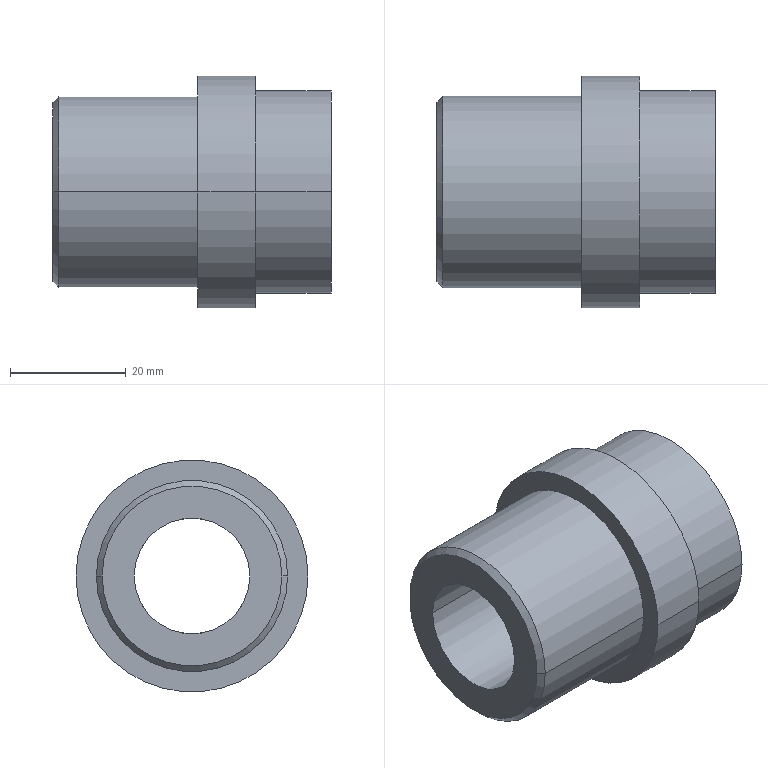Part | SolidWorks | features HoleWzd 1, ICE 1, Revolution 1 | 1 solid | 18 faces | box 48 x 40 x 40 mm | volume 30975 mm3 | cylinder 10 | cone 4 | plane 4 | commonest cylinder face diameters 20 x2 20.5 x2 33 x2 35 x2 40 x2
STEP:
#1=CARTESIAN_POINT('',(-22.,0.,10.25));
#2=VERTEX_POINT('',#1);
#3=CARTESIAN_POINT('',(-22.,0.,-10.25));
#4=VERTEX_POINT('',#3);
#5=CARTESIAN_POINT('',(-22.,0.,0.));
#6=DIRECTION('',(1.,0.,0.));
#7=DIRECTION('',(0.,0.,-1.));
#8=AXIS2_PLACEMENT_3D('',#5,#6,#7);
#9=CIRCLE('',#8,10.25);
#10=EDGE_CURVE('',#2,#4,#9,.T.);
#11=ORIENTED_EDGE('',*,*,#10,.F.);
#12=CARTESIAN_POINT('',(0.,0.,10.25));
#13=VERTEX_POINT('',#12);
#14=CARTESIAN_POINT('',(0.,0.,10.25));
#15=DIRECTION('',(1.,0.,0.));
#16=VECTOR('',#15,1000.);
#17=LINE('',#14,#16);
#18=EDGE_CURVE('',#2,#13,#17,.T.);
#19=ORIENTED_EDGE('',*,*,#18,.T.);
#20=CARTESIAN_POINT('',(0.,0.,-10.25));
#21=VERTEX_POINT('',#20);
#22=CARTESIAN_POINT('',(0.,0.,0.));
#23=DIRECTION('',(1.,0.,0.));
#24=DIRECTION('',(0.,0.,-1.));
#25=AXIS2_PLACEMENT_3D('',#22,#23,#24);
#26=CIRCLE('',#25,10.25);
#27=EDGE_CURVE('',#13,#21,#26,.T.);
#28=ORIENTED_EDGE('',*,*,#27,.T.);
#29=CARTESIAN_POINT('',(0.,0.,-10.25));
#30=DIRECTION('',(1.,0.,0.));
#31=VECTOR('',#30,1000.);
#32=LINE('',#29,#31);
#33=EDGE_CURVE('',#4,#21,#32,.T.);
#34=ORIENTED_EDGE('',*,*,#33,.F.);
#35=EDGE_LOOP('',(#11,#19,#28,#34));
#36=FACE_OUTER_BOUND('',#35,.T.);
#37=CARTESIAN_POINT('',(0.,0.,0.));
#38=DIRECTION('',(1.,0.,0.));
#39=DIRECTION('',(0.,0.,-1.));
#40=AXIS2_PLACEMENT_3D('',#37,#38,#39);
#41=CYLINDRICAL_SURFACE('',#40,10.25);
#42=ADVANCED_FACE('',(#36),#41,.F.);
#43=CARTESIAN_POINT('',(-22.15,0.,10.));
#44=VERTEX_POINT('',#43);
#45=CARTESIAN_POINT('',(-22.15,-10.,0.));
#46=VERTEX_POINT('',#45);
#47=CARTESIAN_POINT('',(-22.15,0.,0.));
#48=DIRECTION('',(1.,0.,0.));
#49=DIRECTION('',(0.,0.,-1.));
#50=AXIS2_PLACEMENT_3D('',#47,#48,#49);
#51=CIRCLE('',#50,10.);
#52=EDGE_CURVE('',#44,#46,#51,.T.);
#53=ORIENTED_EDGE('',*,*,#52,.F.);
#54=CARTESIAN_POINT('',(-22.,0.,10.25));
#55=DIRECTION('',(0.515,0.,0.8572));
#56=VECTOR('',#55,1000.);
#57=LINE('',#54,#56);
#58=EDGE_CURVE('',#44,#2,#57,.T.);
#59=ORIENTED_EDGE('',*,*,#58,.T.);
#60=ORIENTED_EDGE('',*,*,#10,.T.);
#61=CARTESIAN_POINT('',(-22.15,0.,-10.));
#62=VERTEX_POINT('',#61);
#63=CARTESIAN_POINT('',(-22.,0.,-10.25));
#64=DIRECTION('',(0.515,0.,-0.8572));
#65=VECTOR('',#64,1000.);
#66=LINE('',#63,#65);
#67=EDGE_CURVE('',#62,#4,#66,.T.);
#68=ORIENTED_EDGE('',*,*,#67,.F.);
#69=CARTESIAN_POINT('',(-22.15,0.,0.));
#70=DIRECTION('',(1.,0.,0.));
#71=DIRECTION('',(0.,0.,-1.));
#72=AXIS2_PLACEMENT_3D('',#69,#70,#71);
#73=CIRCLE('',#72,10.);
#74=EDGE_CURVE('',#46,#62,#73,.T.);
#75=ORIENTED_EDGE('',*,*,#74,.F.);
#76=EDGE_LOOP('',(#53,#59,#60,#68,#75));
#77=FACE_OUTER_BOUND('',#76,.T.);
#78=CARTESIAN_POINT('',(-22.,0.,0.));
#79=DIRECTION('',(1.,0.,0.));
#80=DIRECTION('',(0.,0.,-1.));
#81=AXIS2_PLACEMENT_3D('',#78,#79,#80);
#82=CONICAL_SURFACE('',#81,10.25,1.03);
#83=ADVANCED_FACE('',(#77),#82,.F.);
#84=CARTESIAN_POINT('',(-48.,-10.,0.));
#85=VERTEX_POINT('',#84);
#86=CARTESIAN_POINT('',(-48.,10.,0.));
#87=VERTEX_POINT('',#86);
#88=CARTESIAN_POINT('',(-48.,0.,0.));
#89=DIRECTION('',(1.,0.,0.));
#90=DIRECTION('',(0.,1.,0.));
#91=AXIS2_PLACEMENT_3D('',#88,#89,#90);
#92=CIRCLE('',#91,10.);
#93=EDGE_CURVE('',#85,#87,#92,.T.);
#94=ORIENTED_EDGE('',*,*,#93,.F.);
#95=CARTESIAN_POINT('',(-48.,-10.,0.));
#96=DIRECTION('',(1.,0.,0.));
#97=VECTOR('',#96,1000.);
#98=LINE('',#95,#97);
#99=EDGE_CURVE('',#85,#46,#98,.T.);
#100=ORIENTED_EDGE('',*,*,#99,.T.);
#101=ORIENTED_EDGE('',*,*,#74,.T.);
#102=CARTESIAN_POINT('',(-22.15,10.,0.));
#103=VERTEX_POINT('',#102);
#104=CARTESIAN_POINT('',(-22.15,0.,0.));
#105=DIRECTION('',(1.,0.,0.));
#106=DIRECTION('',(0.,0.,-1.));
#107=AXIS2_PLACEMENT_3D('',#104,#105,#106);
#108=CIRCLE('',#107,10.);
#109=EDGE_CURVE('',#62,#103,#108,.T.);
#110=ORIENTED_EDGE('',*,*,#109,.T.);
#111=CARTESIAN_POINT('',(-48.,10.,0.));
#112=DIRECTION('',(1.,0.,0.));
#113=VECTOR('',#112,1000.);
#114=LINE('',#111,#113);
#115=EDGE_CURVE('',#87,#103,#114,.T.);
#116=ORIENTED_EDGE('',*,*,#115,.F.);
#117=EDGE_LOOP('',(#94,#100,#101,#110,#116));
#118=FACE_OUTER_BOUND('',#117,.T.);
#119=CARTESIAN_POINT('',(-48.,0.,0.));
#120=DIRECTION('',(1.,0.,0.));
#121=DIRECTION('',(0.,1.,0.));
#122=AXIS2_PLACEMENT_3D('',#119,#120,#121);
#123=CYLINDRICAL_SURFACE('',#122,10.);
#124=ADVANCED_FACE('',(#118),#123,.F.);
#125=CARTESIAN_POINT('',(-13.,17.5,0.));
#126=VERTEX_POINT('',#125);
#127=CARTESIAN_POINT('',(-13.,-17.5,0.));
#128=VERTEX_POINT('',#127);
#129=CARTESIAN_POINT('',(-13.,0.,0.));
#130=DIRECTION('',(1.,0.,0.));
#131=DIRECTION('',(0.,1.,0.));
#132=AXIS2_PLACEMENT_3D('',#129,#130,#131);
#133=CIRCLE('',#132,17.5);
#134=EDGE_CURVE('',#126,#128,#133,.T.);
#135=ORIENTED_EDGE('',*,*,#134,.T.);
#136=CARTESIAN_POINT('',(0.,-17.5,0.));
#137=VERTEX_POINT('',#136);
#138=CARTESIAN_POINT('',(0.,-17.5,0.));
#139=DIRECTION('',(1.,0.,0.));
#140=VECTOR('',#139,1000.);
#141=LINE('',#138,#140);
#142=EDGE_CURVE('',#128,#137,#141,.T.);
#143=ORIENTED_EDGE('',*,*,#142,.T.);
#144=CARTESIAN_POINT('',(0.,17.5,0.));
#145=VERTEX_POINT('',#144);
#146=CARTESIAN_POINT('',(0.,0.,0.));
#147=DIRECTION('',(1.,0.,0.));
#148=DIRECTION('',(0.,1.,0.));
#149=AXIS2_PLACEMENT_3D('',#146,#147,#148);
#150=CIRCLE('',#149,17.5);
#151=EDGE_CURVE('',#145,#137,#150,.T.);
#152=ORIENTED_EDGE('',*,*,#151,.F.);
#153=CARTESIAN_POINT('',(0.,17.5,0.));
#154=DIRECTION('',(1.,0.,0.));
#155=VECTOR('',#154,1000.);
#156=LINE('',#153,#155);
#157=EDGE_CURVE('',#126,#145,#156,.T.);
#158=ORIENTED_EDGE('',*,*,#157,.F.);
#159=EDGE_LOOP('',(#135,#143,#152,#158));
#160=FACE_OUTER_BOUND('',#159,.T.);
#161=CARTESIAN_POINT('',(0.,0.,0.));
#162=DIRECTION('',(1.,0.,0.));
#163=DIRECTION('',(0.,1.,0.));
#164=AXIS2_PLACEMENT_3D('',#161,#162,#163);
#165=CYLINDRICAL_SURFACE('',#164,17.5);
#166=ADVANCED_FACE('',(#160),#165,.T.);
#167=CARTESIAN_POINT('',(-23.,20.,0.));
#168=VERTEX_POINT('',#167);
#169=CARTESIAN_POINT('',(-23.,-20.,0.));
#170=VERTEX_POINT('',#169);
#171=CARTESIAN_POINT('',(-23.,0.,0.));
#172=DIRECTION('',(1.,0.,0.));
#173=DIRECTION('',(0.,1.,0.));
#174=AXIS2_PLACEMENT_3D('',#171,#172,#173);
#175=CIRCLE('',#174,20.);
#176=EDGE_CURVE('',#168,#170,#175,.T.);
#177=ORIENTED_EDGE('',*,*,#176,.T.);
#178=CARTESIAN_POINT('',(-13.,-20.,0.));
#179=VERTEX_POINT('',#178);
#180=CARTESIAN_POINT('',(0.,-20.,0.));
#181=DIRECTION('',(1.,0.,0.));
#182=VECTOR('',#181,1000.);
#183=LINE('',#180,#182);
#184=EDGE_CURVE('',#170,#179,#183,.T.);
#185=ORIENTED_EDGE('',*,*,#184,.T.);
#186=CARTESIAN_POINT('',(-13.,20.,0.));
#187=VERTEX_POINT('',#186);
#188=CARTESIAN_POINT('',(-13.,0.,0.));
#189=DIRECTION('',(1.,0.,0.));
#190=DIRECTION('',(0.,1.,0.));
#191=AXIS2_PLACEMENT_3D('',#188,#189,#190);
#192=CIRCLE('',#191,20.);
#193=EDGE_CURVE('',#187,#179,#192,.T.);
#194=ORIENTED_EDGE('',*,*,#193,.F.);
#195=CARTESIAN_POINT('',(0.,20.,0.));
#196=DIRECTION('',(1.,0.,0.));
#197=VECTOR('',#196,1000.);
#198=LINE('',#195,#197);
#199=EDGE_CURVE('',#168,#187,#198,.T.);
#200=ORIENTED_EDGE('',*,*,#199,.F.);
#201=EDGE_LOOP('',(#177,#185,#194,#200));
#202=FACE_OUTER_BOUND('',#201,.T.);
#203=CARTESIAN_POINT('',(0.,0.,0.));
#204=DIRECTION('',(1.,0.,0.));
#205=DIRECTION('',(0.,1.,0.));
#206=AXIS2_PLACEMENT_3D('',#203,#204,#205);
#207=CYLINDRICAL_SURFACE('',#206,20.);
#208=ADVANCED_FACE('',(#202),#207,.T.);
#209=CARTESIAN_POINT('',(-47.,16.5,0.));
#210=VERTEX_POINT('',#209);
#211=CARTESIAN_POINT('',(-47.,-16.5,0.));
#212=VERTEX_POINT('',#211);
#213=CARTESIAN_POINT('',(-47.,0.,0.));
#214=DIRECTION('',(1.,0.,0.));
#215=DIRECTION('',(0.,1.,0.));
#216=AXIS2_PLACEMENT_3D('',#213,#214,#215);
#217=CIRCLE('',#216,16.5);
#218=EDGE_CURVE('',#210,#212,#217,.T.);
#219=ORIENTED_EDGE('',*,*,#218,.T.);
#220=CARTESIAN_POINT('',(-23.,-16.5,0.));
#221=VERTEX_POINT('',#220);
#222=CARTESIAN_POINT('',(0.,-16.5,0.));
#223=DIRECTION('',(1.,0.,0.));
#224=VECTOR('',#223,1000.);
#225=LINE('',#222,#224);
#226=EDGE_CURVE('',#212,#221,#225,.T.);
#227=ORIENTED_EDGE('',*,*,#226,.T.);
#228=CARTESIAN_POINT('',(-23.,16.5,0.));
#229=VERTEX_POINT('',#228);
#230=CARTESIAN_POINT('',(-23.,0.,0.));
#231=DIRECTION('',(1.,0.,0.));
#232=DIRECTION('',(0.,1.,0.));
#233=AXIS2_PLACEMENT_3D('',#230,#231,#232);
#234=CIRCLE('',#233,16.5);
#235=EDGE_CURVE('',#229,#221,#234,.T.);
#236=ORIENTED_EDGE('',*,*,#235,.F.);
#237=CARTESIAN_POINT('',(0.,16.5,0.));
#238=DIRECTION('',(1.,0.,0.));
#239=VECTOR('',#238,1000.);
#240=LINE('',#237,#239);
#241=EDGE_CURVE('',#210,#229,#240,.T.);
#242=ORIENTED_EDGE('',*,*,#241,.F.);
#243=EDGE_LOOP('',(#219,#227,#236,#242));
#244=FACE_OUTER_BOUND('',#243,.T.);
#245=CARTESIAN_POINT('',(0.,0.,0.));
#246=DIRECTION('',(1.,0.,0.));
#247=DIRECTION('',(0.,1.,0.));
#248=AXIS2_PLACEMENT_3D('',#245,#246,#247);
#249=CYLINDRICAL_SURFACE('',#248,16.5);
#250=ADVANCED_FACE('',(#244),#249,.T.);
#251=CARTESIAN_POINT('',(-48.,15.5,0.));
#252=VERTEX_POINT('',#251);
#253=CARTESIAN_POINT('',(-48.,-15.5,0.));
#254=VERTEX_POINT('',#253);
#255=CARTESIAN_POINT('',(-48.,0.,0.));
#256=DIRECTION('',(1.,0.,0.));
#257=DIRECTION('',(0.,1.,0.));
#258=AXIS2_PLACEMENT_3D('',#255,#256,#257);
#259=CIRCLE('',#258,15.5);
#260=EDGE_CURVE('',#252,#254,#259,.T.);
#261=ORIENTED_EDGE('',*,*,#260,.T.);
#262=CARTESIAN_POINT('',(-47.,-16.5,0.));
#263=DIRECTION('',(0.7071,-0.7071,0.));
#264=VECTOR('',#263,1000.);
#265=LINE('',#262,#264);
#266=EDGE_CURVE('',#254,#212,#265,.T.);
#267=ORIENTED_EDGE('',*,*,#266,.T.);
#268=ORIENTED_EDGE('',*,*,#218,.F.);
#269=CARTESIAN_POINT('',(-47.,16.5,0.));
#270=DIRECTION('',(0.7071,0.7071,0.));
#271=VECTOR('',#270,1000.);
#272=LINE('',#269,#271);
#273=EDGE_CURVE('',#252,#210,#272,.T.);
#274=ORIENTED_EDGE('',*,*,#273,.F.);
#275=EDGE_LOOP('',(#261,#267,#268,#274));
#276=FACE_OUTER_BOUND('',#275,.T.);
#277=CARTESIAN_POINT('',(-47.,0.,0.));
#278=DIRECTION('',(1.,0.,0.));
#279=DIRECTION('',(0.,1.,0.));
#280=AXIS2_PLACEMENT_3D('',#277,#278,#279);
#281=CONICAL_SURFACE('',#280,16.5,0.7854);
#282=ADVANCED_FACE('',(#276),#281,.T.);
#283=CARTESIAN_POINT('',(-48.,0.,0.));
#284=DIRECTION('',(1.,0.,0.));
#285=DIRECTION('',(0.,1.,0.));
#286=AXIS2_PLACEMENT_3D('',#283,#284,#285);
#287=CIRCLE('',#286,10.);
#288=EDGE_CURVE('',#87,#85,#287,.T.);
#289=ORIENTED_EDGE('',*,*,#288,.T.);
#290=ORIENTED_EDGE('',*,*,#93,.T.);
#291=EDGE_LOOP('',(#289,#290));
#292=FACE_BOUND('',#291,.T.);
#293=ORIENTED_EDGE('',*,*,#260,.F.);
#294=CARTESIAN_POINT('',(-48.,0.,0.));
#295=DIRECTION('',(1.,0.,0.));
#296=DIRECTION('',(0.,1.,0.));
#297=AXIS2_PLACEMENT_3D('',#294,#295,#296);
#298=CIRCLE('',#297,15.5);
#299=EDGE_CURVE('',#254,#252,#298,.T.);
#300=ORIENTED_EDGE('',*,*,#299,.F.);
#301=EDGE_LOOP('',(#293,#300));
#302=FACE_OUTER_BOUND('',#301,.T.);
#303=CARTESIAN_POINT('',(-48.,0.,0.));
#304=DIRECTION('',(-1.,0.,0.));
#305=DIRECTION('',(0.,-1.,0.));
#306=AXIS2_PLACEMENT_3D('',#303,#304,#305);
#307=PLANE('',#306);
#308=ADVANCED_FACE('',(#292,#302),#307,.T.);
#309=ORIENTED_EDGE('',*,*,#266,.F.);
#310=ORIENTED_EDGE('',*,*,#299,.T.);
#311=ORIENTED_EDGE('',*,*,#273,.T.);
#312=CARTESIAN_POINT('',(-47.,0.,0.));
#313=DIRECTION('',(1.,0.,0.));
#314=DIRECTION('',(0.,1.,0.));
#315=AXIS2_PLACEMENT_3D('',#312,#313,#314);
#316=CIRCLE('',#315,16.5);
#317=EDGE_CURVE('',#212,#210,#316,.T.);
#318=ORIENTED_EDGE('',*,*,#317,.F.);
#319=EDGE_LOOP('',(#309,#310,#311,#318));
#320=FACE_OUTER_BOUND('',#319,.T.);
#321=CARTESIAN_POINT('',(-47.,0.,0.));
#322=DIRECTION('',(1.,0.,0.));
#323=DIRECTION('',(0.,1.,0.));
#324=AXIS2_PLACEMENT_3D('',#321,#322,#323);
#325=CONICAL_SURFACE('',#324,16.5,0.7854);
#326=ADVANCED_FACE('',(#320),#325,.T.);
#327=ORIENTED_EDGE('',*,*,#226,.F.);
#328=ORIENTED_EDGE('',*,*,#317,.T.);
#329=ORIENTED_EDGE('',*,*,#241,.T.);
#330=CARTESIAN_POINT('',(-23.,0.,0.));
#331=DIRECTION('',(1.,0.,0.));
#332=DIRECTION('',(0.,1.,0.));
#333=AXIS2_PLACEMENT_3D('',#330,#331,#332);
#334=CIRCLE('',#333,16.5);
#335=EDGE_CURVE('',#221,#229,#334,.T.);
#336=ORIENTED_EDGE('',*,*,#335,.F.);
#337=EDGE_LOOP('',(#327,#328,#329,#336));
#338=FACE_OUTER_BOUND('',#337,.T.);
#339=CARTESIAN_POINT('',(0.,0.,0.));
#340=DIRECTION('',(1.,0.,0.));
#341=DIRECTION('',(0.,1.,0.));
#342=AXIS2_PLACEMENT_3D('',#339,#340,#341);
#343=CYLINDRICAL_SURFACE('',#342,16.5);
#344=ADVANCED_FACE('',(#338),#343,.T.);
#345=ORIENTED_EDGE('',*,*,#235,.T.);
#346=ORIENTED_EDGE('',*,*,#335,.T.);
#347=EDGE_LOOP('',(#345,#346));
#348=FACE_BOUND('',#347,.T.);
#349=ORIENTED_EDGE('',*,*,#176,.F.);
#350=CARTESIAN_POINT('',(-23.,0.,0.));
#351=DIRECTION('',(1.,0.,0.));
#352=DIRECTION('',(0.,1.,0.));
#353=AXIS2_PLACEMENT_3D('',#350,#351,#352);
#354=CIRCLE('',#353,20.);
#355=EDGE_CURVE('',#170,#168,#354,.T.);
#356=ORIENTED_EDGE('',*,*,#355,.F.);
#357=EDGE_LOOP('',(#349,#356));
#358=FACE_OUTER_BOUND('',#357,.T.);
#359=CARTESIAN_POINT('',(-23.,16.5,0.));
#360=DIRECTION('',(-1.,0.,0.));
#361=DIRECTION('',(0.,-1.,0.));
#362=AXIS2_PLACEMENT_3D('',#359,#360,#361);
#363=PLANE('',#362);
#364=ADVANCED_FACE('',(#348,#358),#363,.T.);
#365=ORIENTED_EDGE('',*,*,#184,.F.);
#366=ORIENTED_EDGE('',*,*,#355,.T.);
#367=ORIENTED_EDGE('',*,*,#199,.T.);
#368=CARTESIAN_POINT('',(-13.,0.,0.));
#369=DIRECTION('',(1.,0.,0.));
#370=DIRECTION('',(0.,1.,0.));
#371=AXIS2_PLACEMENT_3D('',#368,#369,#370);
#372=CIRCLE('',#371,20.);
#373=EDGE_CURVE('',#179,#187,#372,.T.);
#374=ORIENTED_EDGE('',*,*,#373,.F.);
#375=EDGE_LOOP('',(#365,#366,#367,#374));
#376=FACE_OUTER_BOUND('',#375,.T.);
#377=CARTESIAN_POINT('',(0.,0.,0.));
#378=DIRECTION('',(1.,0.,0.));
#379=DIRECTION('',(0.,1.,0.));
#380=AXIS2_PLACEMENT_3D('',#377,#378,#379);
#381=CYLINDRICAL_SURFACE('',#380,20.);
#382=ADVANCED_FACE('',(#376),#381,.T.);
#383=ORIENTED_EDGE('',*,*,#193,.T.);
#384=ORIENTED_EDGE('',*,*,#373,.T.);
#385=EDGE_LOOP('',(#383,#384));
#386=FACE_OUTER_BOUND('',#385,.T.);
#387=ORIENTED_EDGE('',*,*,#134,.F.);
#388=CARTESIAN_POINT('',(-13.,0.,0.));
#389=DIRECTION('',(1.,0.,0.));
#390=DIRECTION('',(0.,1.,0.));
#391=AXIS2_PLACEMENT_3D('',#388,#389,#390);
#392=CIRCLE('',#391,17.5);
#393=EDGE_CURVE('',#128,#126,#392,.T.);
#394=ORIENTED_EDGE('',*,*,#393,.F.);
#395=EDGE_LOOP('',(#387,#394));
#396=FACE_BOUND('',#395,.T.);
#397=CARTESIAN_POINT('',(-13.,20.,0.));
#398=DIRECTION('',(1.,0.,0.));
#399=DIRECTION('',(0.,1.,0.));
#400=AXIS2_PLACEMENT_3D('',#397,#398,#399);
#401=PLANE('',#400);
#402=ADVANCED_FACE('',(#386,#396),#401,.T.);
#403=ORIENTED_EDGE('',*,*,#142,.F.);
#404=ORIENTED_EDGE('',*,*,#393,.T.);
#405=ORIENTED_EDGE('',*,*,#157,.T.);
#406=CARTESIAN_POINT('',(0.,0.,0.));
#407=DIRECTION('',(1.,0.,0.));
#408=DIRECTION('',(0.,1.,0.));
#409=AXIS2_PLACEMENT_3D('',#406,#407,#408);
#410=CIRCLE('',#409,17.5);
#411=EDGE_CURVE('',#137,#145,#410,.T.);
#412=ORIENTED_EDGE('',*,*,#411,.F.);
#413=EDGE_LOOP('',(#403,#404,#405,#412));
#414=FACE_OUTER_BOUND('',#413,.T.);
#415=CARTESIAN_POINT('',(0.,0.,0.));
#416=DIRECTION('',(1.,0.,0.));
#417=DIRECTION('',(0.,1.,0.));
#418=AXIS2_PLACEMENT_3D('',#415,#416,#417);
#419=CYLINDRICAL_SURFACE('',#418,17.5);
#420=ADVANCED_FACE('',(#414),#419,.T.);
#421=CARTESIAN_POINT('',(0.,0.,0.));
#422=DIRECTION('',(1.,0.,0.));
#423=DIRECTION('',(0.,0.,-1.));
#424=AXIS2_PLACEMENT_3D('',#421,#422,#423);
#425=CIRCLE('',#424,10.25);
#426=EDGE_CURVE('',#21,#13,#425,.T.);
#427=ORIENTED_EDGE('',*,*,#426,.F.);
#428=ORIENTED_EDGE('',*,*,#27,.F.);
#429=EDGE_LOOP('',(#427,#428));
#430=FACE_BOUND('',#429,.T.);
#431=ORIENTED_EDGE('',*,*,#151,.T.);
#432=ORIENTED_EDGE('',*,*,#411,.T.);
#433=EDGE_LOOP('',(#431,#432));
#434=FACE_OUTER_BOUND('',#433,.T.);
#435=CARTESIAN_POINT('',(0.,17.5,0.));
#436=DIRECTION('',(1.,0.,0.));
#437=DIRECTION('',(0.,1.,0.));
#438=AXIS2_PLACEMENT_3D('',#435,#436,#437);
#439=PLANE('',#438);
#440=ADVANCED_FACE('',(#430,#434),#439,.T.);
#441=ORIENTED_EDGE('',*,*,#99,.F.);
#442=ORIENTED_EDGE('',*,*,#288,.F.);
#443=ORIENTED_EDGE('',*,*,#115,.T.);
#444=CARTESIAN_POINT('',(-22.15,0.,0.));
#445=DIRECTION('',(1.,0.,0.));
#446=DIRECTION('',(0.,0.,-1.));
#447=AXIS2_PLACEMENT_3D('',#444,#445,#446);
#448=CIRCLE('',#447,10.);
#449=EDGE_CURVE('',#103,#44,#448,.T.);
#450=ORIENTED_EDGE('',*,*,#449,.T.);
#451=ORIENTED_EDGE('',*,*,#52,.T.);
#452=EDGE_LOOP('',(#441,#442,#443,#450,#451));
#453=FACE_OUTER_BOUND('',#452,.T.);
#454=CARTESIAN_POINT('',(-48.,0.,0.));
#455=DIRECTION('',(1.,0.,0.));
#456=DIRECTION('',(0.,1.,0.));
#457=AXIS2_PLACEMENT_3D('',#454,#455,#456);
#458=CYLINDRICAL_SURFACE('',#457,10.);
#459=ADVANCED_FACE('',(#453),#458,.F.);
#460=ORIENTED_EDGE('',*,*,#58,.F.);
#461=ORIENTED_EDGE('',*,*,#449,.F.);
#462=ORIENTED_EDGE('',*,*,#109,.F.);
#463=ORIENTED_EDGE('',*,*,#67,.T.);
#464=CARTESIAN_POINT('',(-22.,0.,0.));
#465=DIRECTION('',(1.,0.,0.));
#466=DIRECTION('',(0.,0.,-1.));
#467=AXIS2_PLACEMENT_3D('',#464,#465,#466);
#468=CIRCLE('',#467,10.25);
#469=EDGE_CURVE('',#4,#2,#468,.T.);
#470=ORIENTED_EDGE('',*,*,#469,.T.);
#471=EDGE_LOOP('',(#460,#461,#462,#463,#470));
#472=FACE_OUTER_BOUND('',#471,.T.);
#473=CARTESIAN_POINT('',(-22.,0.,0.));
#474=DIRECTION('',(1.,0.,0.));
#475=DIRECTION('',(0.,0.,-1.));
#476=AXIS2_PLACEMENT_3D('',#473,#474,#475);
#477=CONICAL_SURFACE('',#476,10.25,1.03);
#478=ADVANCED_FACE('',(#472),#477,.F.);
#479=ORIENTED_EDGE('',*,*,#18,.F.);
#480=ORIENTED_EDGE('',*,*,#469,.F.);
#481=ORIENTED_EDGE('',*,*,#33,.T.);
#482=ORIENTED_EDGE('',*,*,#426,.T.);
#483=EDGE_LOOP('',(#479,#480,#481,#482));
#484=FACE_OUTER_BOUND('',#483,.T.);
#485=CARTESIAN_POINT('',(0.,0.,0.));
#486=DIRECTION('',(1.,0.,0.));
#487=DIRECTION('',(0.,0.,-1.));
#488=AXIS2_PLACEMENT_3D('',#485,#486,#487);
#489=CYLINDRICAL_SURFACE('',#488,10.25);
#490=ADVANCED_FACE('',(#484),#489,.F.);
#491=CLOSED_SHELL('',(#42,#83,#124,#166,#208,#250,#282,#308,#326,#344,#364,#382,#402,#420,#440,#459,#478,#490));
#492=MANIFOLD_SOLID_BREP('',#491);
#493=CARTESIAN_POINT('',(0.,0.,0.));
#494=DIRECTION('',(0.,0.,1.));
#495=DIRECTION('',(1.,0.,0.));
#496=AXIS2_PLACEMENT_3D('',#493,#494,#495);
#497=(LENGTH_UNIT()NAMED_UNIT(*)SI_UNIT(.MILLI.,.METRE.));
#498=UNCERTAINTY_MEASURE_WITH_UNIT(LENGTH_MEASURE(0.00001),#497,'','');
#499=(NAMED_UNIT(*)PLANE_ANGLE_UNIT()SI_UNIT($,.RADIAN.));
#500=(NAMED_UNIT(*)SI_UNIT($,.STERADIAN.)SOLID_ANGLE_UNIT());
#501=(GEOMETRIC_REPRESENTATION_CONTEXT(3)GLOBAL_UNCERTAINTY_ASSIGNED_CONTEXT((#498))GLOBAL_UNIT_ASSIGNED_CONTEXT((#497,#499,#500))REPRESENTATION_CONTEXT('',''));
#502=ADVANCED_BREP_SHAPE_REPRESENTATION('',(#492,#496),#501);